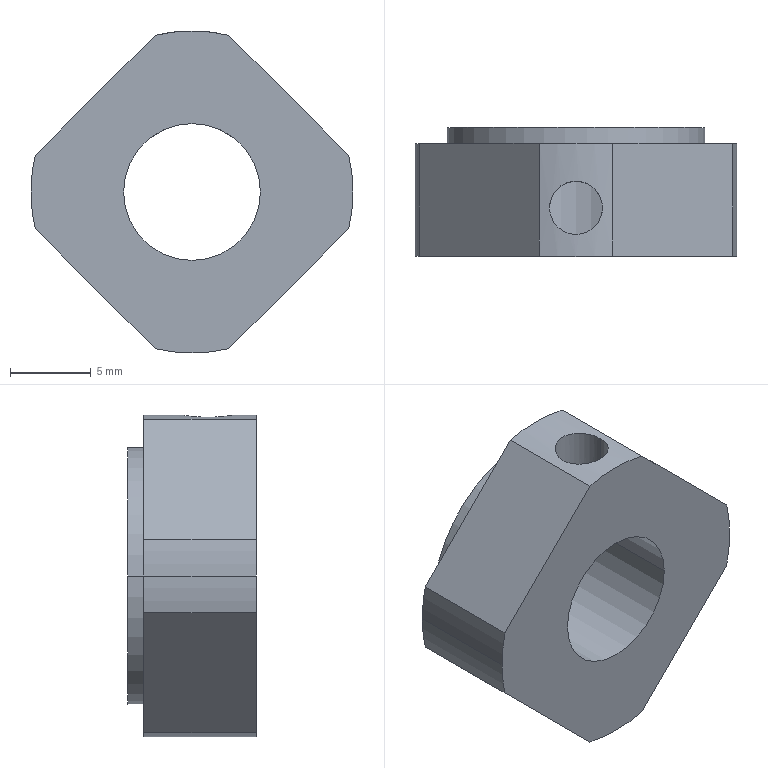Part | NX | 1 solid | 18 faces | box 20 x 8 x 20 mm | volume 1597 mm3 | cylinder 11 | plane 7 | commonest cylinder face diameters 20 x5 3.3 x2 8.5 x2 16 x2
STEP:
#1=CARTESIAN_POINT('',(2.285,0.,-9.735));
#2=VERTEX_POINT('',#1);
#3=CARTESIAN_POINT('',(2.285,7.,-9.735));
#4=VERTEX_POINT('',#3);
#5=CARTESIAN_POINT('',(2.285,0.,-9.735));
#6=DIRECTION('',(0.,1.,0.));
#7=VECTOR('',#6,1000.);
#8=LINE('',#5,#7);
#9=EDGE_CURVE('',#2,#4,#8,.T.);
#10=ORIENTED_EDGE('',*,*,#9,.F.);
#11=CARTESIAN_POINT('',(-2.285,0.,-9.735));
#12=VERTEX_POINT('',#11);
#13=CARTESIAN_POINT('',(0.,0.,0.));
#14=DIRECTION('',(0.,1.,0.));
#15=DIRECTION('',(0.2285,0.,-0.9735));
#16=AXIS2_PLACEMENT_3D('',#13,#14,#15);
#17=CIRCLE('',#16,10.);
#18=EDGE_CURVE('',#2,#12,#17,.T.);
#19=ORIENTED_EDGE('',*,*,#18,.T.);
#20=CARTESIAN_POINT('',(-2.285,7.,-9.735));
#21=VERTEX_POINT('',#20);
#22=CARTESIAN_POINT('',(-2.285,7.,-9.735));
#23=DIRECTION('',(0.,-1.,0.));
#24=VECTOR('',#23,1000.);
#25=LINE('',#22,#24);
#26=EDGE_CURVE('',#21,#12,#25,.T.);
#27=ORIENTED_EDGE('',*,*,#26,.F.);
#28=CARTESIAN_POINT('',(0.,7.,0.));
#29=DIRECTION('',(0.,-1.,0.));
#30=DIRECTION('',(-0.2285,0.,-0.9735));
#31=AXIS2_PLACEMENT_3D('',#28,#29,#30);
#32=CIRCLE('',#31,10.);
#33=EDGE_CURVE('',#21,#4,#32,.T.);
#34=ORIENTED_EDGE('',*,*,#33,.T.);
#35=EDGE_LOOP('',(#10,#19,#27,#34));
#36=FACE_BOUND('',#35,.T.);
#37=CARTESIAN_POINT('',(0.,8.4,0.));
#38=DIRECTION('',(0.,-1.,0.));
#39=DIRECTION('',(-1.,0.,0.));
#40=AXIS2_PLACEMENT_3D('',#37,#38,#39);
#41=CYLINDRICAL_SURFACE('',#40,10.);
#42=ADVANCED_FACE('',(#36),#41,.T.);
#43=ORIENTED_EDGE('',*,*,#9,.T.);
#44=CARTESIAN_POINT('',(9.735,7.,-2.285));
#45=VERTEX_POINT('',#44);
#46=CARTESIAN_POINT('',(2.285,7.,-9.735));
#47=DIRECTION('',(0.7071,0.,0.7071));
#48=VECTOR('',#47,1000.);
#49=LINE('',#46,#48);
#50=EDGE_CURVE('',#4,#45,#49,.T.);
#51=ORIENTED_EDGE('',*,*,#50,.T.);
#52=CARTESIAN_POINT('',(9.735,0.,-2.285));
#53=VERTEX_POINT('',#52);
#54=CARTESIAN_POINT('',(9.735,7.,-2.285));
#55=DIRECTION('',(0.,-1.,0.));
#56=VECTOR('',#55,1000.);
#57=LINE('',#54,#56);
#58=EDGE_CURVE('',#45,#53,#57,.T.);
#59=ORIENTED_EDGE('',*,*,#58,.T.);
#60=CARTESIAN_POINT('',(9.735,0.,-2.285));
#61=DIRECTION('',(-0.7071,0.,-0.7071));
#62=VECTOR('',#61,1000.);
#63=LINE('',#60,#62);
#64=EDGE_CURVE('',#53,#2,#63,.T.);
#65=ORIENTED_EDGE('',*,*,#64,.T.);
#66=EDGE_LOOP('',(#43,#51,#59,#65));
#67=FACE_BOUND('',#66,.T.);
#68=CARTESIAN_POINT('',(0.,7.,-12.021));
#69=DIRECTION('',(-0.7071,0.,0.7071));
#70=DIRECTION('',(0.,1.,0.));
#71=AXIS2_PLACEMENT_3D('',#68,#69,#70);
#72=PLANE('',#71);
#73=ADVANCED_FACE('',(#67),#72,.F.);
#74=ORIENTED_EDGE('',*,*,#64,.F.);
#75=CARTESIAN_POINT('',(9.735,0.,2.285));
#76=VERTEX_POINT('',#75);
#77=CARTESIAN_POINT('',(0.,0.,0.));
#78=DIRECTION('',(0.,1.,0.));
#79=DIRECTION('',(1.,0.,0.));
#80=AXIS2_PLACEMENT_3D('',#77,#78,#79);
#81=CIRCLE('',#80,10.);
#82=EDGE_CURVE('',#76,#53,#81,.T.);
#83=ORIENTED_EDGE('',*,*,#82,.F.);
#84=CARTESIAN_POINT('',(2.285,0.,9.735));
#85=VERTEX_POINT('',#84);
#86=CARTESIAN_POINT('',(2.285,0.,9.735));
#87=DIRECTION('',(0.7071,0.,-0.7071));
#88=VECTOR('',#87,1000.);
#89=LINE('',#86,#88);
#90=EDGE_CURVE('',#85,#76,#89,.T.);
#91=ORIENTED_EDGE('',*,*,#90,.F.);
#92=CARTESIAN_POINT('',(-2.285,0.,9.735));
#93=VERTEX_POINT('',#92);
#94=CARTESIAN_POINT('',(0.,0.,0.));
#95=DIRECTION('',(0.,1.,0.));
#96=DIRECTION('',(-0.2285,0.,0.9735));
#97=AXIS2_PLACEMENT_3D('',#94,#95,#96);
#98=CIRCLE('',#97,10.);
#99=EDGE_CURVE('',#93,#85,#98,.T.);
#100=ORIENTED_EDGE('',*,*,#99,.F.);
#101=CARTESIAN_POINT('',(-9.735,0.,2.285));
#102=VERTEX_POINT('',#101);
#103=CARTESIAN_POINT('',(-9.735,0.,2.285));
#104=DIRECTION('',(0.7071,0.,0.7071));
#105=VECTOR('',#104,1000.);
#106=LINE('',#103,#105);
#107=EDGE_CURVE('',#102,#93,#106,.T.);
#108=ORIENTED_EDGE('',*,*,#107,.F.);
#109=CARTESIAN_POINT('',(-10.,0.,0.));
#110=VERTEX_POINT('',#109);
#111=CARTESIAN_POINT('',(0.,0.,0.));
#112=DIRECTION('',(0.,1.,0.));
#113=DIRECTION('',(-1.,0.,0.));
#114=AXIS2_PLACEMENT_3D('',#111,#112,#113);
#115=CIRCLE('',#114,10.);
#116=EDGE_CURVE('',#110,#102,#115,.T.);
#117=ORIENTED_EDGE('',*,*,#116,.F.);
#118=CARTESIAN_POINT('',(-9.735,0.,-2.285));
#119=VERTEX_POINT('',#118);
#120=CARTESIAN_POINT('',(0.,0.,0.));
#121=DIRECTION('',(0.,1.,0.));
#122=DIRECTION('',(-1.,0.,0.));
#123=AXIS2_PLACEMENT_3D('',#120,#121,#122);
#124=CIRCLE('',#123,10.);
#125=EDGE_CURVE('',#119,#110,#124,.T.);
#126=ORIENTED_EDGE('',*,*,#125,.F.);
#127=CARTESIAN_POINT('',(-2.285,0.,-9.735));
#128=DIRECTION('',(-0.7071,0.,0.7071));
#129=VECTOR('',#128,1000.);
#130=LINE('',#127,#129);
#131=EDGE_CURVE('',#12,#119,#130,.T.);
#132=ORIENTED_EDGE('',*,*,#131,.F.);
#133=ORIENTED_EDGE('',*,*,#18,.F.);
#134=EDGE_LOOP('',(#74,#83,#91,#100,#108,#117,#126,#132,#133));
#135=FACE_BOUND('',#134,.T.);
#136=CARTESIAN_POINT('',(-4.25,0.,0.));
#137=VERTEX_POINT('',#136);
#138=CARTESIAN_POINT('',(4.25,0.,0.));
#139=VERTEX_POINT('',#138);
#140=CARTESIAN_POINT('',(0.,0.,0.));
#141=DIRECTION('',(0.,-1.,0.));
#142=DIRECTION('',(1.,0.,0.));
#143=AXIS2_PLACEMENT_3D('',#140,#141,#142);
#144=CIRCLE('',#143,4.25);
#145=EDGE_CURVE('',#137,#139,#144,.T.);
#146=ORIENTED_EDGE('',*,*,#145,.F.);
#147=CARTESIAN_POINT('',(0.,0.,0.));
#148=DIRECTION('',(0.,-1.,0.));
#149=DIRECTION('',(1.,0.,0.));
#150=AXIS2_PLACEMENT_3D('',#147,#148,#149);
#151=CIRCLE('',#150,4.25);
#152=EDGE_CURVE('',#139,#137,#151,.T.);
#153=ORIENTED_EDGE('',*,*,#152,.F.);
#154=EDGE_LOOP('',(#146,#153));
#155=FACE_BOUND('',#154,.T.);
#156=CARTESIAN_POINT('',(0.,0.,0.));
#157=DIRECTION('',(0.,-1.,0.));
#158=DIRECTION('',(0.,0.,-1.));
#159=AXIS2_PLACEMENT_3D('',#156,#157,#158);
#160=PLANE('',#159);
#161=ADVANCED_FACE('',(#135,#155),#160,.T.);
#162=CARTESIAN_POINT('',(-9.735,7.,-2.285));
#163=VERTEX_POINT('',#162);
#164=CARTESIAN_POINT('',(-9.735,0.,-2.285));
#165=DIRECTION('',(0.,1.,0.));
#166=VECTOR('',#165,1000.);
#167=LINE('',#164,#166);
#168=EDGE_CURVE('',#119,#163,#167,.T.);
#169=ORIENTED_EDGE('',*,*,#168,.T.);
#170=CARTESIAN_POINT('',(-9.735,7.,-2.285));
#171=DIRECTION('',(0.7071,0.,-0.7071));
#172=VECTOR('',#171,1000.);
#173=LINE('',#170,#172);
#174=EDGE_CURVE('',#163,#21,#173,.T.);
#175=ORIENTED_EDGE('',*,*,#174,.T.);
#176=ORIENTED_EDGE('',*,*,#26,.T.);
#177=ORIENTED_EDGE('',*,*,#131,.T.);
#178=EDGE_LOOP('',(#169,#175,#176,#177));
#179=FACE_BOUND('',#178,.T.);
#180=CARTESIAN_POINT('',(-12.021,7.,0.));
#181=DIRECTION('',(0.7071,0.,0.7071));
#182=DIRECTION('',(0.,-1.,0.));
#183=AXIS2_PLACEMENT_3D('',#180,#181,#182);
#184=PLANE('',#183);
#185=ADVANCED_FACE('',(#179),#184,.F.);
#186=CARTESIAN_POINT('',(-10.,7.,0.));
#187=VERTEX_POINT('',#186);
#188=CARTESIAN_POINT('',(-10.,8.4,0.));
#189=DIRECTION('',(0.,-1.,0.));
#190=VECTOR('',#189,1000.);
#191=LINE('',#188,#190);
#192=EDGE_CURVE('',#187,#110,#191,.T.);
#193=ORIENTED_EDGE('',*,*,#192,.F.);
#194=CARTESIAN_POINT('',(0.,7.,0.));
#195=DIRECTION('',(0.,-1.,0.));
#196=DIRECTION('',(-0.9735,0.,0.2285));
#197=AXIS2_PLACEMENT_3D('',#194,#195,#196);
#198=CIRCLE('',#197,10.);
#199=EDGE_CURVE('',#187,#163,#198,.T.);
#200=ORIENTED_EDGE('',*,*,#199,.T.);
#201=ORIENTED_EDGE('',*,*,#168,.F.);
#202=ORIENTED_EDGE('',*,*,#125,.T.);
#203=EDGE_LOOP('',(#193,#200,#201,#202));
#204=FACE_BOUND('',#203,.T.);
#205=CARTESIAN_POINT('',(0.,8.4,0.));
#206=DIRECTION('',(0.,-1.,0.));
#207=DIRECTION('',(-1.,0.,0.));
#208=AXIS2_PLACEMENT_3D('',#205,#206,#207);
#209=CYLINDRICAL_SURFACE('',#208,10.);
#210=ADVANCED_FACE('',(#204),#209,.T.);
#211=ORIENTED_EDGE('',*,*,#50,.F.);
#212=ORIENTED_EDGE('',*,*,#33,.F.);
#213=ORIENTED_EDGE('',*,*,#174,.F.);
#214=ORIENTED_EDGE('',*,*,#199,.F.);
#215=CARTESIAN_POINT('',(-9.735,7.,2.285));
#216=VERTEX_POINT('',#215);
#217=CARTESIAN_POINT('',(0.,7.,0.));
#218=DIRECTION('',(0.,-1.,0.));
#219=DIRECTION('',(-0.9735,0.,0.2285));
#220=AXIS2_PLACEMENT_3D('',#217,#218,#219);
#221=CIRCLE('',#220,10.);
#222=EDGE_CURVE('',#216,#187,#221,.T.);
#223=ORIENTED_EDGE('',*,*,#222,.F.);
#224=CARTESIAN_POINT('',(-2.285,7.,9.735));
#225=VERTEX_POINT('',#224);
#226=CARTESIAN_POINT('',(-2.285,7.,9.735));
#227=DIRECTION('',(-0.7071,0.,-0.7071));
#228=VECTOR('',#227,1000.);
#229=LINE('',#226,#228);
#230=EDGE_CURVE('',#225,#216,#229,.T.);
#231=ORIENTED_EDGE('',*,*,#230,.F.);
#232=CARTESIAN_POINT('',(2.285,7.,9.735));
#233=VERTEX_POINT('',#232);
#234=CARTESIAN_POINT('',(0.,7.,0.));
#235=DIRECTION('',(0.,-1.,0.));
#236=DIRECTION('',(0.2285,0.,0.9735));
#237=AXIS2_PLACEMENT_3D('',#234,#235,#236);
#238=CIRCLE('',#237,10.);
#239=EDGE_CURVE('',#233,#225,#238,.T.);
#240=ORIENTED_EDGE('',*,*,#239,.F.);
#241=CARTESIAN_POINT('',(9.735,7.,2.285));
#242=VERTEX_POINT('',#241);
#243=CARTESIAN_POINT('',(9.735,7.,2.285));
#244=DIRECTION('',(-0.7071,0.,0.7071));
#245=VECTOR('',#244,1000.);
#246=LINE('',#243,#245);
#247=EDGE_CURVE('',#242,#233,#246,.T.);
#248=ORIENTED_EDGE('',*,*,#247,.F.);
#249=CARTESIAN_POINT('',(0.,7.,0.));
#250=DIRECTION('',(0.,-1.,0.));
#251=DIRECTION('',(1.,0.,0.));
#252=AXIS2_PLACEMENT_3D('',#249,#250,#251);
#253=CIRCLE('',#252,10.);
#254=EDGE_CURVE('',#45,#242,#253,.T.);
#255=ORIENTED_EDGE('',*,*,#254,.F.);
#256=EDGE_LOOP('',(#211,#212,#213,#214,#223,#231,#240,#248,#255));
#257=FACE_BOUND('',#256,.T.);
#258=CARTESIAN_POINT('',(8.,7.,0.));
#259=VERTEX_POINT('',#258);
#260=CARTESIAN_POINT('',(-8.,7.,0.));
#261=VERTEX_POINT('',#260);
#262=CARTESIAN_POINT('',(0.,7.,0.));
#263=DIRECTION('',(0.,1.,0.));
#264=DIRECTION('',(1.,0.,0.));
#265=AXIS2_PLACEMENT_3D('',#262,#263,#264);
#266=CIRCLE('',#265,8.);
#267=EDGE_CURVE('',#259,#261,#266,.T.);
#268=ORIENTED_EDGE('',*,*,#267,.F.);
#269=CARTESIAN_POINT('',(0.,7.,0.));
#270=DIRECTION('',(0.,1.,0.));
#271=DIRECTION('',(1.,0.,0.));
#272=AXIS2_PLACEMENT_3D('',#269,#270,#271);
#273=CIRCLE('',#272,8.);
#274=EDGE_CURVE('',#261,#259,#273,.T.);
#275=ORIENTED_EDGE('',*,*,#274,.F.);
#276=EDGE_LOOP('',(#268,#275));
#277=FACE_BOUND('',#276,.T.);
#278=CARTESIAN_POINT('',(0.,7.,0.));
#279=DIRECTION('',(0.,-1.,0.));
#280=DIRECTION('',(0.,0.,-1.));
#281=AXIS2_PLACEMENT_3D('',#278,#279,#280);
#282=PLANE('',#281);
#283=ADVANCED_FACE('',(#257,#277),#282,.F.);
#284=ORIENTED_EDGE('',*,*,#254,.T.);
#285=CARTESIAN_POINT('',(9.735,0.,2.285));
#286=DIRECTION('',(0.,1.,0.));
#287=VECTOR('',#286,1000.);
#288=LINE('',#285,#287);
#289=EDGE_CURVE('',#76,#242,#288,.T.);
#290=ORIENTED_EDGE('',*,*,#289,.F.);
#291=ORIENTED_EDGE('',*,*,#82,.T.);
#292=ORIENTED_EDGE('',*,*,#58,.F.);
#293=EDGE_LOOP('',(#284,#290,#291,#292));
#294=FACE_BOUND('',#293,.T.);
#295=CARTESIAN_POINT('',(0.,8.4,0.));
#296=DIRECTION('',(0.,-1.,0.));
#297=DIRECTION('',(-1.,0.,0.));
#298=AXIS2_PLACEMENT_3D('',#295,#296,#297);
#299=CYLINDRICAL_SURFACE('',#298,10.);
#300=ADVANCED_FACE('',(#294),#299,.T.);
#301=ORIENTED_EDGE('',*,*,#289,.T.);
#302=ORIENTED_EDGE('',*,*,#247,.T.);
#303=CARTESIAN_POINT('',(2.285,7.,9.735));
#304=DIRECTION('',(0.,-1.,0.));
#305=VECTOR('',#304,1000.);
#306=LINE('',#303,#305);
#307=EDGE_CURVE('',#233,#85,#306,.T.);
#308=ORIENTED_EDGE('',*,*,#307,.T.);
#309=ORIENTED_EDGE('',*,*,#90,.T.);
#310=EDGE_LOOP('',(#301,#302,#308,#309));
#311=FACE_BOUND('',#310,.T.);
#312=CARTESIAN_POINT('',(12.021,7.,0.));
#313=DIRECTION('',(-0.7071,0.,-0.7071));
#314=DIRECTION('',(-0.7071,0.,0.7071));
#315=AXIS2_PLACEMENT_3D('',#312,#313,#314);
#316=PLANE('',#315);
#317=ADVANCED_FACE('',(#311),#316,.F.);
#318=ORIENTED_EDGE('',*,*,#307,.F.);
#319=ORIENTED_EDGE('',*,*,#239,.T.);
#320=CARTESIAN_POINT('',(-2.285,0.,9.735));
#321=DIRECTION('',(0.,1.,0.));
#322=VECTOR('',#321,1000.);
#323=LINE('',#320,#322);
#324=EDGE_CURVE('',#93,#225,#323,.T.);
#325=ORIENTED_EDGE('',*,*,#324,.F.);
#326=ORIENTED_EDGE('',*,*,#99,.T.);
#327=EDGE_LOOP('',(#318,#319,#325,#326));
#328=FACE_BOUND('',#327,.T.);
#329=CARTESIAN_POINT('',(-1.65,3.,9.863));
#330=VERTEX_POINT('',#329);
#331=CARTESIAN_POINT('',(1.65,3.,9.863));
#332=VERTEX_POINT('',#331);
#333=CARTESIAN_POINT('',(-1.65,3.,9.863));
#334=CARTESIAN_POINT('',(-1.65,3.433,9.863));
#335=CARTESIAN_POINT('',(-1.302,4.283,9.931));
#336=CARTESIAN_POINT('',(0.001859,4.831,10.034));
#337=CARTESIAN_POINT('',(1.288,4.295,9.932));
#338=CARTESIAN_POINT('',(1.65,3.437,9.863));
#339=CARTESIAN_POINT('',(1.65,3.,9.863));
#340=B_SPLINE_CURVE_WITH_KNOTS('',3,(#333,#334,#335,#336,#337,#338,#339),.UNSPECIFIED.,.F.,.F.,(4,1,1,1,4),(0.,0.25,0.5,0.75,1.),.UNSPECIFIED.);
#341=EDGE_CURVE('',#330,#332,#340,.T.);
#342=ORIENTED_EDGE('',*,*,#341,.T.);
#343=CARTESIAN_POINT('',(1.65,3.,9.863));
#344=CARTESIAN_POINT('',(1.65,2.567,9.863));
#345=CARTESIAN_POINT('',(1.302,1.717,9.931));
#346=CARTESIAN_POINT('',(-0.001862,1.169,10.034));
#347=CARTESIAN_POINT('',(-1.288,1.705,9.932));
#348=CARTESIAN_POINT('',(-1.65,2.563,9.863));
#349=CARTESIAN_POINT('',(-1.65,3.,9.863));
#350=B_SPLINE_CURVE_WITH_KNOTS('',3,(#343,#344,#345,#346,#347,#348,#349),.UNSPECIFIED.,.F.,.F.,(4,1,1,1,4),(0.,0.25,0.5,0.75,1.),.UNSPECIFIED.);
#351=EDGE_CURVE('',#332,#330,#350,.T.);
#352=ORIENTED_EDGE('',*,*,#351,.T.);
#353=EDGE_LOOP('',(#342,#352));
#354=FACE_BOUND('',#353,.T.);
#355=CARTESIAN_POINT('',(0.,8.4,0.));
#356=DIRECTION('',(0.,-1.,0.));
#357=DIRECTION('',(-1.,0.,0.));
#358=AXIS2_PLACEMENT_3D('',#355,#356,#357);
#359=CYLINDRICAL_SURFACE('',#358,10.);
#360=ADVANCED_FACE('',(#328,#354),#359,.T.);
#361=ORIENTED_EDGE('',*,*,#324,.T.);
#362=ORIENTED_EDGE('',*,*,#230,.T.);
#363=CARTESIAN_POINT('',(-9.735,7.,2.285));
#364=DIRECTION('',(0.,-1.,0.));
#365=VECTOR('',#364,1000.);
#366=LINE('',#363,#365);
#367=EDGE_CURVE('',#216,#102,#366,.T.);
#368=ORIENTED_EDGE('',*,*,#367,.T.);
#369=ORIENTED_EDGE('',*,*,#107,.T.);
#370=EDGE_LOOP('',(#361,#362,#368,#369));
#371=FACE_BOUND('',#370,.T.);
#372=CARTESIAN_POINT('',(0.,7.,12.021));
#373=DIRECTION('',(0.7071,0.,-0.7071));
#374=DIRECTION('',(0.,-1.,0.));
#375=AXIS2_PLACEMENT_3D('',#372,#373,#374);
#376=PLANE('',#375);
#377=ADVANCED_FACE('',(#371),#376,.F.);
#378=CARTESIAN_POINT('',(-1.65,3.,3.917));
#379=VERTEX_POINT('',#378);
#380=CARTESIAN_POINT('',(1.65,3.,3.917));
#381=VERTEX_POINT('',#380);
#382=CARTESIAN_POINT('',(-1.65,3.,3.917));
#383=CARTESIAN_POINT('',(-1.65,3.198,3.917));
#384=CARTESIAN_POINT('',(-1.559,3.581,3.954));
#385=CARTESIAN_POINT('',(-1.434,3.834,4.003));
#386=CARTESIAN_POINT('',(-1.182,4.18,4.086));
#387=CARTESIAN_POINT('',(-0.8751,4.408,4.161));
#388=CARTESIAN_POINT('',(-0.5935,4.555,4.214));
#389=CARTESIAN_POINT('',(-0.03899,4.706,4.271));
#390=CARTESIAN_POINT('',(0.5445,4.575,4.221));
#391=CARTESIAN_POINT('',(0.8516,4.425,4.166));
#392=CARTESIAN_POINT('',(1.186,4.178,4.086));
#393=CARTESIAN_POINT('',(1.44,3.826,4.001));
#394=CARTESIAN_POINT('',(1.569,3.557,3.95));
#395=CARTESIAN_POINT('',(1.65,3.193,3.917));
#396=CARTESIAN_POINT('',(1.65,3.,3.917));
#397=B_SPLINE_CURVE_WITH_KNOTS('',3,(#382,#383,#384,#385,#386,#387,#388,#389,#390,#391,#392,#393,#394,#395,#396),.UNSPECIFIED.,.F.,.F.,(4,1,1,1,1,1,1,1,1,1,1,1,4),(0.,0.125,0.1875,0.25,0.3125,0.375,0.5,0.625,0.6875,0.75,0.8125,0.875,1.),.UNSPECIFIED.);
#398=EDGE_CURVE('',#379,#381,#397,.T.);
#399=ORIENTED_EDGE('',*,*,#398,.T.);
#400=CARTESIAN_POINT('',(1.65,3.,10.));
#401=DIRECTION('',(0.,0.,-1.));
#402=VECTOR('',#401,1000.);
#403=LINE('',#400,#402);
#404=EDGE_CURVE('',#381,#332,#403,.F.);
#405=ORIENTED_EDGE('',*,*,#404,.T.);
#406=ORIENTED_EDGE('',*,*,#341,.F.);
#407=CARTESIAN_POINT('',(-1.65,3.,10.));
#408=DIRECTION('',(0.,0.,-1.));
#409=VECTOR('',#408,1000.);
#410=LINE('',#407,#409);
#411=EDGE_CURVE('',#379,#330,#410,.F.);
#412=ORIENTED_EDGE('',*,*,#411,.F.);
#413=EDGE_LOOP('',(#399,#405,#406,#412));
#414=FACE_BOUND('',#413,.T.);
#415=CARTESIAN_POINT('',(0.,3.,10.));
#416=DIRECTION('',(0.,0.,-1.));
#417=DIRECTION('',(-1.,0.,0.));
#418=AXIS2_PLACEMENT_3D('',#415,#416,#417);
#419=CYLINDRICAL_SURFACE('',#418,1.65);
#420=ADVANCED_FACE('',(#414),#419,.F.);
#421=ORIENTED_EDGE('',*,*,#267,.T.);
#422=CARTESIAN_POINT('',(-8.,8.,0.));
#423=VERTEX_POINT('',#422);
#424=CARTESIAN_POINT('',(-8.,8.4,0.));
#425=DIRECTION('',(0.,-1.,0.));
#426=VECTOR('',#425,1000.);
#427=LINE('',#424,#426);
#428=EDGE_CURVE('',#261,#423,#427,.F.);
#429=ORIENTED_EDGE('',*,*,#428,.T.);
#430=CARTESIAN_POINT('',(8.,8.,0.));
#431=VERTEX_POINT('',#430);
#432=CARTESIAN_POINT('',(0.,8.,0.));
#433=DIRECTION('',(0.,-1.,0.));
#434=DIRECTION('',(1.,0.,0.));
#435=AXIS2_PLACEMENT_3D('',#432,#433,#434);
#436=CIRCLE('',#435,8.);
#437=EDGE_CURVE('',#423,#431,#436,.T.);
#438=ORIENTED_EDGE('',*,*,#437,.T.);
#439=CARTESIAN_POINT('',(8.,8.4,0.));
#440=DIRECTION('',(0.,-1.,0.));
#441=VECTOR('',#440,1000.);
#442=LINE('',#439,#441);
#443=EDGE_CURVE('',#259,#431,#442,.F.);
#444=ORIENTED_EDGE('',*,*,#443,.F.);
#445=EDGE_LOOP('',(#421,#429,#438,#444));
#446=FACE_BOUND('',#445,.T.);
#447=CARTESIAN_POINT('',(0.,8.4,0.));
#448=DIRECTION('',(0.,-1.,0.));
#449=DIRECTION('',(-1.,0.,0.));
#450=AXIS2_PLACEMENT_3D('',#447,#448,#449);
#451=CYLINDRICAL_SURFACE('',#450,8.);
#452=ADVANCED_FACE('',(#446),#451,.T.);
#453=CARTESIAN_POINT('',(4.25,8.,0.));
#454=VERTEX_POINT('',#453);
#455=CARTESIAN_POINT('',(-4.25,8.,0.));
#456=VERTEX_POINT('',#455);
#457=CARTESIAN_POINT('',(0.,8.,0.));
#458=DIRECTION('',(0.,1.,0.));
#459=DIRECTION('',(-1.,0.,0.));
#460=AXIS2_PLACEMENT_3D('',#457,#458,#459);
#461=CIRCLE('',#460,4.25);
#462=EDGE_CURVE('',#454,#456,#461,.T.);
#463=ORIENTED_EDGE('',*,*,#462,.T.);
#464=CARTESIAN_POINT('',(-4.25,8.4,0.));
#465=DIRECTION('',(0.,-1.,0.));
#466=VECTOR('',#465,1000.);
#467=LINE('',#464,#466);
#468=EDGE_CURVE('',#137,#456,#467,.F.);
#469=ORIENTED_EDGE('',*,*,#468,.F.);
#470=ORIENTED_EDGE('',*,*,#145,.T.);
#471=CARTESIAN_POINT('',(4.25,8.4,0.));
#472=DIRECTION('',(0.,-1.,0.));
#473=VECTOR('',#472,1000.);
#474=LINE('',#471,#473);
#475=EDGE_CURVE('',#139,#454,#474,.F.);
#476=ORIENTED_EDGE('',*,*,#475,.T.);
#477=EDGE_LOOP('',(#463,#469,#470,#476));
#478=FACE_BOUND('',#477,.T.);
#479=CARTESIAN_POINT('',(0.,8.4,0.));
#480=DIRECTION('',(0.,-1.,0.));
#481=DIRECTION('',(-1.,0.,0.));
#482=AXIS2_PLACEMENT_3D('',#479,#480,#481);
#483=CYLINDRICAL_SURFACE('',#482,4.25);
#484=ADVANCED_FACE('',(#478),#483,.F.);
#485=ORIENTED_EDGE('',*,*,#437,.F.);
#486=CARTESIAN_POINT('',(0.,8.,0.));
#487=DIRECTION('',(0.,-1.,0.));
#488=DIRECTION('',(1.,0.,0.));
#489=AXIS2_PLACEMENT_3D('',#486,#487,#488);
#490=CIRCLE('',#489,8.);
#491=EDGE_CURVE('',#431,#423,#490,.T.);
#492=ORIENTED_EDGE('',*,*,#491,.F.);
#493=EDGE_LOOP('',(#485,#492));
#494=FACE_BOUND('',#493,.T.);
#495=ORIENTED_EDGE('',*,*,#462,.F.);
#496=CARTESIAN_POINT('',(0.,8.,0.));
#497=DIRECTION('',(0.,1.,0.));
#498=DIRECTION('',(-1.,0.,0.));
#499=AXIS2_PLACEMENT_3D('',#496,#497,#498);
#500=CIRCLE('',#499,4.25);
#501=EDGE_CURVE('',#456,#454,#500,.T.);
#502=ORIENTED_EDGE('',*,*,#501,.F.);
#503=EDGE_LOOP('',(#495,#502));
#504=FACE_BOUND('',#503,.T.);
#505=CARTESIAN_POINT('',(0.,8.,0.));
#506=DIRECTION('',(0.,-1.,0.));
#507=DIRECTION('',(0.,0.,-1.));
#508=AXIS2_PLACEMENT_3D('',#505,#506,#507);
#509=PLANE('',#508);
#510=ADVANCED_FACE('',(#494,#504),#509,.F.);
#511=ORIENTED_EDGE('',*,*,#411,.T.);
#512=ORIENTED_EDGE('',*,*,#351,.F.);
#513=ORIENTED_EDGE('',*,*,#404,.F.);
#514=CARTESIAN_POINT('',(1.65,3.,3.917));
#515=CARTESIAN_POINT('',(1.65,2.802,3.917));
#516=CARTESIAN_POINT('',(1.559,2.417,3.954));
#517=CARTESIAN_POINT('',(1.434,2.165,4.003));
#518=CARTESIAN_POINT('',(1.182,1.82,4.086));
#519=CARTESIAN_POINT('',(0.8757,1.592,4.161));
#520=CARTESIAN_POINT('',(0.5946,1.445,4.214));
#521=CARTESIAN_POINT('',(0.04037,1.294,4.271));
#522=CARTESIAN_POINT('',(-0.5433,1.424,4.222));
#523=CARTESIAN_POINT('',(-0.8507,1.575,4.166));
#524=CARTESIAN_POINT('',(-1.184,1.82,4.086));
#525=CARTESIAN_POINT('',(-1.439,2.173,4.001));
#526=CARTESIAN_POINT('',(-1.568,2.441,3.95));
#527=CARTESIAN_POINT('',(-1.65,2.806,3.917));
#528=CARTESIAN_POINT('',(-1.65,3.,3.917));
#529=B_SPLINE_CURVE_WITH_KNOTS('',3,(#514,#515,#516,#517,#518,#519,#520,#521,#522,#523,#524,#525,#526,#527,#528),.UNSPECIFIED.,.F.,.F.,(4,1,1,1,1,1,1,1,1,1,1,1,4),(0.,0.125,0.1875,0.25,0.3125,0.375,0.5,0.625,0.6875,0.75,0.8125,0.875,1.),.UNSPECIFIED.);
#530=EDGE_CURVE('',#381,#379,#529,.T.);
#531=ORIENTED_EDGE('',*,*,#530,.T.);
#532=EDGE_LOOP('',(#511,#512,#513,#531));
#533=FACE_BOUND('',#532,.T.);
#534=CARTESIAN_POINT('',(0.,3.,10.));
#535=DIRECTION('',(0.,0.,-1.));
#536=DIRECTION('',(-1.,0.,0.));
#537=AXIS2_PLACEMENT_3D('',#534,#535,#536);
#538=CYLINDRICAL_SURFACE('',#537,1.65);
#539=ADVANCED_FACE('',(#533),#538,.F.);
#540=ORIENTED_EDGE('',*,*,#468,.T.);
#541=ORIENTED_EDGE('',*,*,#501,.T.);
#542=ORIENTED_EDGE('',*,*,#475,.F.);
#543=ORIENTED_EDGE('',*,*,#152,.T.);
#544=EDGE_LOOP('',(#540,#541,#542,#543));
#545=FACE_BOUND('',#544,.T.);
#546=ORIENTED_EDGE('',*,*,#398,.F.);
#547=ORIENTED_EDGE('',*,*,#530,.F.);
#548=EDGE_LOOP('',(#546,#547));
#549=FACE_BOUND('',#548,.T.);
#550=CARTESIAN_POINT('',(0.,8.4,0.));
#551=DIRECTION('',(0.,-1.,0.));
#552=DIRECTION('',(-1.,0.,0.));
#553=AXIS2_PLACEMENT_3D('',#550,#551,#552);
#554=CYLINDRICAL_SURFACE('',#553,4.25);
#555=ADVANCED_FACE('',(#545,#549),#554,.F.);
#556=ORIENTED_EDGE('',*,*,#428,.F.);
#557=ORIENTED_EDGE('',*,*,#274,.T.);
#558=ORIENTED_EDGE('',*,*,#443,.T.);
#559=ORIENTED_EDGE('',*,*,#491,.T.);
#560=EDGE_LOOP('',(#556,#557,#558,#559));
#561=FACE_BOUND('',#560,.T.);
#562=CARTESIAN_POINT('',(0.,8.4,0.));
#563=DIRECTION('',(0.,-1.,0.));
#564=DIRECTION('',(-1.,0.,0.));
#565=AXIS2_PLACEMENT_3D('',#562,#563,#564);
#566=CYLINDRICAL_SURFACE('',#565,8.);
#567=ADVANCED_FACE('',(#561),#566,.T.);
#568=ORIENTED_EDGE('',*,*,#222,.T.);
#569=ORIENTED_EDGE('',*,*,#192,.T.);
#570=ORIENTED_EDGE('',*,*,#116,.T.);
#571=ORIENTED_EDGE('',*,*,#367,.F.);
#572=EDGE_LOOP('',(#568,#569,#570,#571));
#573=FACE_BOUND('',#572,.T.);
#574=CARTESIAN_POINT('',(0.,8.4,0.));
#575=DIRECTION('',(0.,-1.,0.));
#576=DIRECTION('',(-1.,0.,0.));
#577=AXIS2_PLACEMENT_3D('',#574,#575,#576);
#578=CYLINDRICAL_SURFACE('',#577,10.);
#579=ADVANCED_FACE('',(#573),#578,.T.);
#580=CLOSED_SHELL('',(#42,#73,#161,#185,#210,#283,#300,#317,#360,#377,#420,#452,#484,#510,#539,#555,#567,#579));
#581=MANIFOLD_SOLID_BREP('',#580);
#582=(LENGTH_UNIT()NAMED_UNIT(*)SI_UNIT(.MILLI.,.METRE.));
#583=UNCERTAINTY_MEASURE_WITH_UNIT(LENGTH_MEASURE(0.0508),#582,'','');
#584=(NAMED_UNIT(*)PLANE_ANGLE_UNIT()SI_UNIT($,.RADIAN.));
#585=(NAMED_UNIT(*)SI_UNIT($,.STERADIAN.)SOLID_ANGLE_UNIT());
#586=(GEOMETRIC_REPRESENTATION_CONTEXT(3)GLOBAL_UNCERTAINTY_ASSIGNED_CONTEXT((#583))GLOBAL_UNIT_ASSIGNED_CONTEXT((#582,#584,#585))REPRESENTATION_CONTEXT('',''));
#587=ADVANCED_BREP_SHAPE_REPRESENTATION('',(#581),#586);